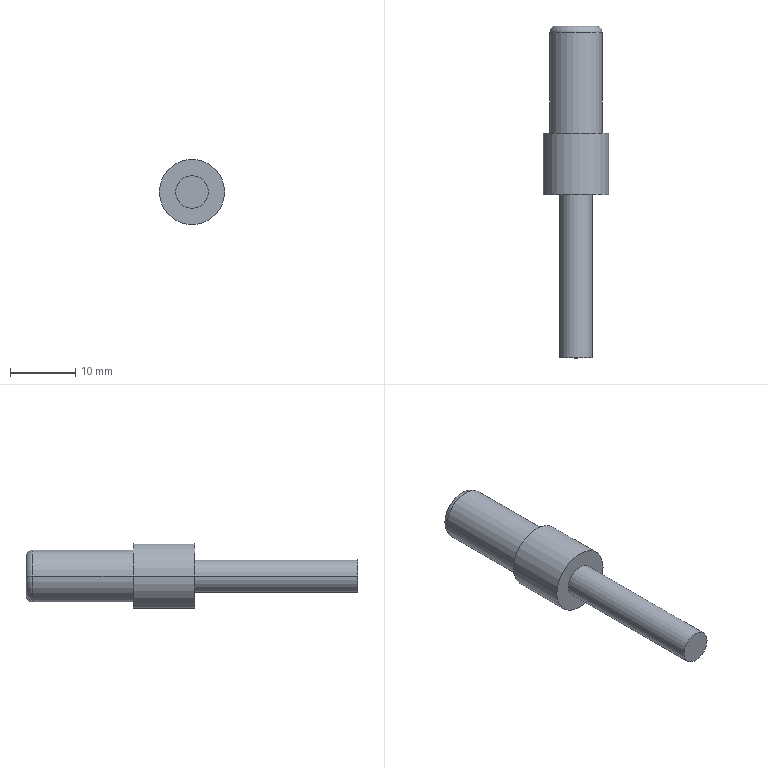Part | STEP file | 11-NEZIPART_CLDM5-25-B11 | 1 solid | 19 faces | box 10 x 50.8 x 10 mm | volume 2025 mm3 | plane 11 | cylinder 6 | torus 2 | commonest cylinder face diameters 5 x2 8 x2 10 x2
STEP:
#1=CARTESIAN_POINT('',(-2.5,-25.,0.));
#2=VERTEX_POINT('',#1);
#3=CARTESIAN_POINT('',(2.5,-25.,0.));
#4=VERTEX_POINT('',#3);
#5=CARTESIAN_POINT('',(0.,-25.,0.));
#6=DIRECTION('',(0.,1.,0.));
#7=DIRECTION('',(-1.,0.,0.));
#8=AXIS2_PLACEMENT_3D('',#5,#6,#7);
#9=CIRCLE('',#8,2.5);
#10=EDGE_CURVE('',#2,#4,#9,.T.);
#11=ORIENTED_EDGE('',*,*,#10,.T.);
#12=CARTESIAN_POINT('',(2.5,0.,0.));
#13=VERTEX_POINT('',#12);
#14=CARTESIAN_POINT('',(2.5,25.8,0.));
#15=DIRECTION('',(0.,1.,0.));
#16=VECTOR('',#15,1000.);
#17=LINE('',#14,#16);
#18=EDGE_CURVE('',#4,#13,#17,.T.);
#19=ORIENTED_EDGE('',*,*,#18,.T.);
#20=CARTESIAN_POINT('',(-2.5,0.,0.));
#21=VERTEX_POINT('',#20);
#22=CARTESIAN_POINT('',(0.,0.,0.));
#23=DIRECTION('',(0.,1.,0.));
#24=DIRECTION('',(-1.,0.,0.));
#25=AXIS2_PLACEMENT_3D('',#22,#23,#24);
#26=CIRCLE('',#25,2.5);
#27=EDGE_CURVE('',#21,#13,#26,.T.);
#28=ORIENTED_EDGE('',*,*,#27,.F.);
#29=CARTESIAN_POINT('',(-2.5,25.8,0.));
#30=DIRECTION('',(0.,1.,0.));
#31=VECTOR('',#30,1000.);
#32=LINE('',#29,#31);
#33=EDGE_CURVE('',#2,#21,#32,.T.);
#34=ORIENTED_EDGE('',*,*,#33,.F.);
#35=EDGE_LOOP('',(#11,#19,#28,#34));
#36=FACE_OUTER_BOUND('',#35,.T.);
#37=CARTESIAN_POINT('',(0.,25.8,0.));
#38=DIRECTION('',(0.,1.,0.));
#39=DIRECTION('',(-1.,0.,0.));
#40=AXIS2_PLACEMENT_3D('',#37,#38,#39);
#41=CYLINDRICAL_SURFACE('',#40,2.5);
#42=ADVANCED_FACE('',(#36),#41,.T.);
#43=CARTESIAN_POINT('',(-4.,24.8,0.));
#44=VERTEX_POINT('',#43);
#45=CARTESIAN_POINT('',(4.,24.8,0.));
#46=VERTEX_POINT('',#45);
#47=CARTESIAN_POINT('',(0.,24.8,0.));
#48=DIRECTION('',(0.,1.,0.));
#49=DIRECTION('',(-1.,0.,0.));
#50=AXIS2_PLACEMENT_3D('',#47,#48,#49);
#51=CIRCLE('',#50,4.);
#52=EDGE_CURVE('',#44,#46,#51,.T.);
#53=ORIENTED_EDGE('',*,*,#52,.T.);
#54=CARTESIAN_POINT('',(3.,25.8,0.));
#55=VERTEX_POINT('',#54);
#56=CARTESIAN_POINT('',(3.,24.8,0.));
#57=DIRECTION('',(0.,0.,1.));
#58=DIRECTION('',(1.,0.,0.));
#59=AXIS2_PLACEMENT_3D('',#56,#57,#58);
#60=CIRCLE('',#59,1.);
#61=EDGE_CURVE('',#46,#55,#60,.T.);
#62=ORIENTED_EDGE('',*,*,#61,.T.);
#63=CARTESIAN_POINT('',(-3.,25.8,0.));
#64=VERTEX_POINT('',#63);
#65=CARTESIAN_POINT('',(0.,25.8,0.));
#66=DIRECTION('',(0.,1.,0.));
#67=DIRECTION('',(-1.,0.,0.));
#68=AXIS2_PLACEMENT_3D('',#65,#66,#67);
#69=CIRCLE('',#68,3.);
#70=EDGE_CURVE('',#64,#55,#69,.T.);
#71=ORIENTED_EDGE('',*,*,#70,.F.);
#72=CARTESIAN_POINT('',(-3.,24.8,0.));
#73=DIRECTION('',(0.,0.,-1.));
#74=DIRECTION('',(-1.,0.,0.));
#75=AXIS2_PLACEMENT_3D('',#72,#73,#74);
#76=CIRCLE('',#75,1.);
#77=EDGE_CURVE('',#44,#64,#76,.T.);
#78=ORIENTED_EDGE('',*,*,#77,.F.);
#79=EDGE_LOOP('',(#53,#62,#71,#78));
#80=FACE_OUTER_BOUND('',#79,.T.);
#81=CARTESIAN_POINT('',(0.,24.8,0.));
#82=DIRECTION('',(0.,1.,0.));
#83=DIRECTION('',(-1.,0.,0.));
#84=AXIS2_PLACEMENT_3D('',#81,#82,#83);
#85=TOROIDAL_SURFACE('',#84,3.,1.);
#86=ADVANCED_FACE('',(#80),#85,.T.);
#87=CARTESIAN_POINT('',(-4.,9.4,0.));
#88=VERTEX_POINT('',#87);
#89=CARTESIAN_POINT('',(4.,9.4,0.));
#90=VERTEX_POINT('',#89);
#91=CARTESIAN_POINT('',(0.,9.4,0.));
#92=DIRECTION('',(0.,1.,0.));
#93=DIRECTION('',(-1.,0.,0.));
#94=AXIS2_PLACEMENT_3D('',#91,#92,#93);
#95=CIRCLE('',#94,4.);
#96=EDGE_CURVE('',#88,#90,#95,.T.);
#97=ORIENTED_EDGE('',*,*,#96,.T.);
#98=CARTESIAN_POINT('',(4.,25.8,0.));
#99=DIRECTION('',(0.,1.,0.));
#100=VECTOR('',#99,1000.);
#101=LINE('',#98,#100);
#102=EDGE_CURVE('',#90,#46,#101,.T.);
#103=ORIENTED_EDGE('',*,*,#102,.T.);
#104=ORIENTED_EDGE('',*,*,#52,.F.);
#105=CARTESIAN_POINT('',(-4.,25.8,0.));
#106=DIRECTION('',(0.,1.,0.));
#107=VECTOR('',#106,1000.);
#108=LINE('',#105,#107);
#109=EDGE_CURVE('',#88,#44,#108,.T.);
#110=ORIENTED_EDGE('',*,*,#109,.F.);
#111=EDGE_LOOP('',(#97,#103,#104,#110));
#112=FACE_OUTER_BOUND('',#111,.T.);
#113=CARTESIAN_POINT('',(0.,25.8,0.));
#114=DIRECTION('',(0.,1.,0.));
#115=DIRECTION('',(-1.,0.,0.));
#116=AXIS2_PLACEMENT_3D('',#113,#114,#115);
#117=CYLINDRICAL_SURFACE('',#116,4.);
#118=ADVANCED_FACE('',(#112),#117,.T.);
#119=CARTESIAN_POINT('',(-5.,0.,0.));
#120=VERTEX_POINT('',#119);
#121=CARTESIAN_POINT('',(5.,0.,0.));
#122=VERTEX_POINT('',#121);
#123=CARTESIAN_POINT('',(0.,0.,0.));
#124=DIRECTION('',(0.,1.,0.));
#125=DIRECTION('',(-1.,0.,0.));
#126=AXIS2_PLACEMENT_3D('',#123,#124,#125);
#127=CIRCLE('',#126,5.);
#128=EDGE_CURVE('',#120,#122,#127,.T.);
#129=ORIENTED_EDGE('',*,*,#128,.T.);
#130=CARTESIAN_POINT('',(5.,9.4,0.));
#131=VERTEX_POINT('',#130);
#132=CARTESIAN_POINT('',(5.,25.8,0.));
#133=DIRECTION('',(0.,1.,0.));
#134=VECTOR('',#133,1000.);
#135=LINE('',#132,#134);
#136=EDGE_CURVE('',#122,#131,#135,.T.);
#137=ORIENTED_EDGE('',*,*,#136,.T.);
#138=CARTESIAN_POINT('',(-5.,9.4,0.));
#139=VERTEX_POINT('',#138);
#140=CARTESIAN_POINT('',(0.,9.4,0.));
#141=DIRECTION('',(0.,1.,0.));
#142=DIRECTION('',(-1.,0.,0.));
#143=AXIS2_PLACEMENT_3D('',#140,#141,#142);
#144=CIRCLE('',#143,5.);
#145=EDGE_CURVE('',#139,#131,#144,.T.);
#146=ORIENTED_EDGE('',*,*,#145,.F.);
#147=CARTESIAN_POINT('',(-5.,25.8,0.));
#148=DIRECTION('',(0.,1.,0.));
#149=VECTOR('',#148,1000.);
#150=LINE('',#147,#149);
#151=EDGE_CURVE('',#120,#139,#150,.T.);
#152=ORIENTED_EDGE('',*,*,#151,.F.);
#153=EDGE_LOOP('',(#129,#137,#146,#152));
#154=FACE_OUTER_BOUND('',#153,.T.);
#155=CARTESIAN_POINT('',(0.,25.8,0.));
#156=DIRECTION('',(0.,1.,0.));
#157=DIRECTION('',(-1.,0.,0.));
#158=AXIS2_PLACEMENT_3D('',#155,#156,#157);
#159=CYLINDRICAL_SURFACE('',#158,5.);
#160=ADVANCED_FACE('',(#154),#159,.T.);
#161=ORIENTED_EDGE('',*,*,#128,.F.);
#162=CARTESIAN_POINT('',(0.,0.,0.));
#163=DIRECTION('',(0.,1.,0.));
#164=DIRECTION('',(-1.,0.,0.));
#165=AXIS2_PLACEMENT_3D('',#162,#163,#164);
#166=CIRCLE('',#165,5.);
#167=EDGE_CURVE('',#122,#120,#166,.T.);
#168=ORIENTED_EDGE('',*,*,#167,.F.);
#169=EDGE_LOOP('',(#161,#168));
#170=FACE_OUTER_BOUND('',#169,.T.);
#171=ORIENTED_EDGE('',*,*,#27,.T.);
#172=CARTESIAN_POINT('',(0.,0.,0.));
#173=DIRECTION('',(0.,1.,0.));
#174=DIRECTION('',(-1.,0.,0.));
#175=AXIS2_PLACEMENT_3D('',#172,#173,#174);
#176=CIRCLE('',#175,2.5);
#177=EDGE_CURVE('',#13,#21,#176,.T.);
#178=ORIENTED_EDGE('',*,*,#177,.T.);
#179=EDGE_LOOP('',(#171,#178));
#180=FACE_BOUND('',#179,.T.);
#181=CARTESIAN_POINT('',(2.5,0.,0.));
#182=DIRECTION('',(0.,1.,0.));
#183=DIRECTION('',(-1.,0.,0.));
#184=AXIS2_PLACEMENT_3D('',#181,#182,#183);
#185=PLANE('',#184);
#186=ADVANCED_FACE('',(#170,#180),#185,.F.);
#187=ORIENTED_EDGE('',*,*,#136,.F.);
#188=ORIENTED_EDGE('',*,*,#167,.T.);
#189=ORIENTED_EDGE('',*,*,#151,.T.);
#190=CARTESIAN_POINT('',(0.,9.4,0.));
#191=DIRECTION('',(0.,1.,0.));
#192=DIRECTION('',(-1.,0.,0.));
#193=AXIS2_PLACEMENT_3D('',#190,#191,#192);
#194=CIRCLE('',#193,5.);
#195=EDGE_CURVE('',#131,#139,#194,.T.);
#196=ORIENTED_EDGE('',*,*,#195,.F.);
#197=EDGE_LOOP('',(#187,#188,#189,#196));
#198=FACE_OUTER_BOUND('',#197,.T.);
#199=CARTESIAN_POINT('',(0.,25.8,0.));
#200=DIRECTION('',(0.,1.,0.));
#201=DIRECTION('',(-1.,0.,0.));
#202=AXIS2_PLACEMENT_3D('',#199,#200,#201);
#203=CYLINDRICAL_SURFACE('',#202,5.);
#204=ADVANCED_FACE('',(#198),#203,.T.);
#205=ORIENTED_EDGE('',*,*,#96,.F.);
#206=CARTESIAN_POINT('',(0.,9.4,0.));
#207=DIRECTION('',(0.,1.,0.));
#208=DIRECTION('',(-1.,0.,0.));
#209=AXIS2_PLACEMENT_3D('',#206,#207,#208);
#210=CIRCLE('',#209,4.);
#211=EDGE_CURVE('',#90,#88,#210,.T.);
#212=ORIENTED_EDGE('',*,*,#211,.F.);
#213=EDGE_LOOP('',(#205,#212));
#214=FACE_BOUND('',#213,.T.);
#215=ORIENTED_EDGE('',*,*,#145,.T.);
#216=ORIENTED_EDGE('',*,*,#195,.T.);
#217=EDGE_LOOP('',(#215,#216));
#218=FACE_OUTER_BOUND('',#217,.T.);
#219=CARTESIAN_POINT('',(5.,9.4,0.));
#220=DIRECTION('',(0.,-1.,0.));
#221=DIRECTION('',(1.,0.,0.));
#222=AXIS2_PLACEMENT_3D('',#219,#220,#221);
#223=PLANE('',#222);
#224=ADVANCED_FACE('',(#214,#218),#223,.F.);
#225=ORIENTED_EDGE('',*,*,#102,.F.);
#226=ORIENTED_EDGE('',*,*,#211,.T.);
#227=ORIENTED_EDGE('',*,*,#109,.T.);
#228=CARTESIAN_POINT('',(0.,24.8,0.));
#229=DIRECTION('',(0.,1.,0.));
#230=DIRECTION('',(-1.,0.,0.));
#231=AXIS2_PLACEMENT_3D('',#228,#229,#230);
#232=CIRCLE('',#231,4.);
#233=EDGE_CURVE('',#46,#44,#232,.T.);
#234=ORIENTED_EDGE('',*,*,#233,.F.);
#235=EDGE_LOOP('',(#225,#226,#227,#234));
#236=FACE_OUTER_BOUND('',#235,.T.);
#237=CARTESIAN_POINT('',(0.,25.8,0.));
#238=DIRECTION('',(0.,1.,0.));
#239=DIRECTION('',(-1.,0.,0.));
#240=AXIS2_PLACEMENT_3D('',#237,#238,#239);
#241=CYLINDRICAL_SURFACE('',#240,4.);
#242=ADVANCED_FACE('',(#236),#241,.T.);
#243=ORIENTED_EDGE('',*,*,#61,.F.);
#244=ORIENTED_EDGE('',*,*,#233,.T.);
#245=ORIENTED_EDGE('',*,*,#77,.T.);
#246=CARTESIAN_POINT('',(0.,25.8,0.));
#247=DIRECTION('',(0.,1.,0.));
#248=DIRECTION('',(-1.,0.,0.));
#249=AXIS2_PLACEMENT_3D('',#246,#247,#248);
#250=CIRCLE('',#249,3.);
#251=EDGE_CURVE('',#55,#64,#250,.T.);
#252=ORIENTED_EDGE('',*,*,#251,.F.);
#253=EDGE_LOOP('',(#243,#244,#245,#252));
#254=FACE_OUTER_BOUND('',#253,.T.);
#255=CARTESIAN_POINT('',(0.,24.8,0.));
#256=DIRECTION('',(0.,1.,0.));
#257=DIRECTION('',(-1.,0.,0.));
#258=AXIS2_PLACEMENT_3D('',#255,#256,#257);
#259=TOROIDAL_SURFACE('',#258,3.,1.);
#260=ADVANCED_FACE('',(#254),#259,.T.);
#261=CARTESIAN_POINT('',(0.,25.8,-1.732));
#262=VERTEX_POINT('',#261);
#263=CARTESIAN_POINT('',(-1.5,25.8,-0.866));
#264=VERTEX_POINT('',#263);
#265=CARTESIAN_POINT('',(0.,25.8,-1.732));
#266=DIRECTION('',(-0.866,0.,0.5));
#267=VECTOR('',#266,1000.);
#268=LINE('',#265,#267);
#269=EDGE_CURVE('',#262,#264,#268,.T.);
#270=ORIENTED_EDGE('',*,*,#269,.F.);
#271=CARTESIAN_POINT('',(1.5,25.8,-0.866));
#272=VERTEX_POINT('',#271);
#273=CARTESIAN_POINT('',(1.5,25.8,-0.866));
#274=DIRECTION('',(-0.866,0.,-0.5));
#275=VECTOR('',#274,1000.);
#276=LINE('',#273,#275);
#277=EDGE_CURVE('',#272,#262,#276,.T.);
#278=ORIENTED_EDGE('',*,*,#277,.F.);
#279=CARTESIAN_POINT('',(1.5,25.8,0.866));
#280=VERTEX_POINT('',#279);
#281=CARTESIAN_POINT('',(1.5,25.8,0.866));
#282=DIRECTION('',(0.,0.,-1.));
#283=VECTOR('',#282,1000.);
#284=LINE('',#281,#283);
#285=EDGE_CURVE('',#280,#272,#284,.T.);
#286=ORIENTED_EDGE('',*,*,#285,.F.);
#287=CARTESIAN_POINT('',(0.,25.8,1.732));
#288=VERTEX_POINT('',#287);
#289=CARTESIAN_POINT('',(0.,25.8,1.732));
#290=DIRECTION('',(0.866,0.,-0.5));
#291=VECTOR('',#290,1000.);
#292=LINE('',#289,#291);
#293=EDGE_CURVE('',#288,#280,#292,.T.);
#294=ORIENTED_EDGE('',*,*,#293,.F.);
#295=CARTESIAN_POINT('',(-1.5,25.8,0.866));
#296=VERTEX_POINT('',#295);
#297=CARTESIAN_POINT('',(-1.5,25.8,0.866));
#298=DIRECTION('',(0.866,0.,0.5));
#299=VECTOR('',#298,1000.);
#300=LINE('',#297,#299);
#301=EDGE_CURVE('',#296,#288,#300,.T.);
#302=ORIENTED_EDGE('',*,*,#301,.F.);
#303=CARTESIAN_POINT('',(-1.5,25.8,-0.866));
#304=DIRECTION('',(0.,0.,1.));
#305=VECTOR('',#304,1000.);
#306=LINE('',#303,#305);
#307=EDGE_CURVE('',#264,#296,#306,.T.);
#308=ORIENTED_EDGE('',*,*,#307,.F.);
#309=EDGE_LOOP('',(#270,#278,#286,#294,#302,#308));
#310=FACE_BOUND('',#309,.T.);
#311=ORIENTED_EDGE('',*,*,#70,.T.);
#312=ORIENTED_EDGE('',*,*,#251,.T.);
#313=EDGE_LOOP('',(#311,#312));
#314=FACE_OUTER_BOUND('',#313,.T.);
#315=CARTESIAN_POINT('',(3.,25.8,0.));
#316=DIRECTION('',(0.,-1.,0.));
#317=DIRECTION('',(1.,0.,0.));
#318=AXIS2_PLACEMENT_3D('',#315,#316,#317);
#319=PLANE('',#318);
#320=ADVANCED_FACE('',(#310,#314),#319,.F.);
#321=ORIENTED_EDGE('',*,*,#10,.F.);
#322=CARTESIAN_POINT('',(0.,-25.,0.));
#323=DIRECTION('',(0.,1.,0.));
#324=DIRECTION('',(-1.,0.,0.));
#325=AXIS2_PLACEMENT_3D('',#322,#323,#324);
#326=CIRCLE('',#325,2.5);
#327=EDGE_CURVE('',#4,#2,#326,.T.);
#328=ORIENTED_EDGE('',*,*,#327,.F.);
#329=EDGE_LOOP('',(#321,#328));
#330=FACE_OUTER_BOUND('',#329,.T.);
#331=CARTESIAN_POINT('',(0.,-25.,0.));
#332=DIRECTION('',(0.,1.,0.));
#333=DIRECTION('',(-1.,0.,0.));
#334=AXIS2_PLACEMENT_3D('',#331,#332,#333);
#335=PLANE('',#334);
#336=ADVANCED_FACE('',(#330),#335,.F.);
#337=ORIENTED_EDGE('',*,*,#18,.F.);
#338=ORIENTED_EDGE('',*,*,#327,.T.);
#339=ORIENTED_EDGE('',*,*,#33,.T.);
#340=ORIENTED_EDGE('',*,*,#177,.F.);
#341=EDGE_LOOP('',(#337,#338,#339,#340));
#342=FACE_OUTER_BOUND('',#341,.T.);
#343=CARTESIAN_POINT('',(0.,25.8,0.));
#344=DIRECTION('',(0.,1.,0.));
#345=DIRECTION('',(-1.,0.,0.));
#346=AXIS2_PLACEMENT_3D('',#343,#344,#345);
#347=CYLINDRICAL_SURFACE('',#346,2.5);
#348=ADVANCED_FACE('',(#342),#347,.T.);
#349=ORIENTED_EDGE('',*,*,#277,.T.);
#350=CARTESIAN_POINT('',(0.,22.8,-1.732));
#351=VERTEX_POINT('',#350);
#352=CARTESIAN_POINT('',(0.,22.8,-1.732));
#353=DIRECTION('',(0.,1.,0.));
#354=VECTOR('',#353,1000.);
#355=LINE('',#352,#354);
#356=EDGE_CURVE('',#351,#262,#355,.T.);
#357=ORIENTED_EDGE('',*,*,#356,.F.);
#358=CARTESIAN_POINT('',(1.5,22.8,-0.866));
#359=VERTEX_POINT('',#358);
#360=CARTESIAN_POINT('',(1.5,22.8,-0.866));
#361=DIRECTION('',(-0.866,0.,-0.5));
#362=VECTOR('',#361,1000.);
#363=LINE('',#360,#362);
#364=EDGE_CURVE('',#359,#351,#363,.T.);
#365=ORIENTED_EDGE('',*,*,#364,.F.);
#366=CARTESIAN_POINT('',(1.5,22.8,-0.866));
#367=DIRECTION('',(0.,1.,0.));
#368=VECTOR('',#367,1000.);
#369=LINE('',#366,#368);
#370=EDGE_CURVE('',#359,#272,#369,.T.);
#371=ORIENTED_EDGE('',*,*,#370,.T.);
#372=EDGE_LOOP('',(#349,#357,#365,#371));
#373=FACE_OUTER_BOUND('',#372,.T.);
#374=CARTESIAN_POINT('',(1.5,22.8,-0.866));
#375=DIRECTION('',(0.5,0.,-0.866));
#376=DIRECTION('',(-0.866,0.,-0.5));
#377=AXIS2_PLACEMENT_3D('',#374,#375,#376);
#378=PLANE('',#377);
#379=ADVANCED_FACE('',(#373),#378,.F.);
#380=ORIENTED_EDGE('',*,*,#285,.T.);
#381=ORIENTED_EDGE('',*,*,#370,.F.);
#382=CARTESIAN_POINT('',(1.5,22.8,0.866));
#383=VERTEX_POINT('',#382);
#384=CARTESIAN_POINT('',(1.5,22.8,0.866));
#385=DIRECTION('',(0.,0.,-1.));
#386=VECTOR('',#385,1000.);
#387=LINE('',#384,#386);
#388=EDGE_CURVE('',#383,#359,#387,.T.);
#389=ORIENTED_EDGE('',*,*,#388,.F.);
#390=CARTESIAN_POINT('',(1.5,22.8,0.866));
#391=DIRECTION('',(0.,1.,0.));
#392=VECTOR('',#391,1000.);
#393=LINE('',#390,#392);
#394=EDGE_CURVE('',#383,#280,#393,.T.);
#395=ORIENTED_EDGE('',*,*,#394,.T.);
#396=EDGE_LOOP('',(#380,#381,#389,#395));
#397=FACE_OUTER_BOUND('',#396,.T.);
#398=CARTESIAN_POINT('',(1.5,22.8,0.866));
#399=DIRECTION('',(1.,0.,0.));
#400=DIRECTION('',(0.,0.,-1.));
#401=AXIS2_PLACEMENT_3D('',#398,#399,#400);
#402=PLANE('',#401);
#403=ADVANCED_FACE('',(#397),#402,.F.);
#404=ORIENTED_EDGE('',*,*,#293,.T.);
#405=ORIENTED_EDGE('',*,*,#394,.F.);
#406=CARTESIAN_POINT('',(0.,22.8,1.732));
#407=VERTEX_POINT('',#406);
#408=CARTESIAN_POINT('',(0.,22.8,1.732));
#409=DIRECTION('',(0.866,0.,-0.5));
#410=VECTOR('',#409,1000.);
#411=LINE('',#408,#410);
#412=EDGE_CURVE('',#407,#383,#411,.T.);
#413=ORIENTED_EDGE('',*,*,#412,.F.);
#414=CARTESIAN_POINT('',(0.,22.8,1.732));
#415=DIRECTION('',(0.,1.,0.));
#416=VECTOR('',#415,1000.);
#417=LINE('',#414,#416);
#418=EDGE_CURVE('',#407,#288,#417,.T.);
#419=ORIENTED_EDGE('',*,*,#418,.T.);
#420=EDGE_LOOP('',(#404,#405,#413,#419));
#421=FACE_OUTER_BOUND('',#420,.T.);
#422=CARTESIAN_POINT('',(0.,22.8,1.732));
#423=DIRECTION('',(0.5,0.,0.866));
#424=DIRECTION('',(0.866,0.,-0.5));
#425=AXIS2_PLACEMENT_3D('',#422,#423,#424);
#426=PLANE('',#425);
#427=ADVANCED_FACE('',(#421),#426,.F.);
#428=ORIENTED_EDGE('',*,*,#301,.T.);
#429=ORIENTED_EDGE('',*,*,#418,.F.);
#430=CARTESIAN_POINT('',(-1.5,22.8,0.866));
#431=VERTEX_POINT('',#430);
#432=CARTESIAN_POINT('',(-1.5,22.8,0.866));
#433=DIRECTION('',(0.866,0.,0.5));
#434=VECTOR('',#433,1000.);
#435=LINE('',#432,#434);
#436=EDGE_CURVE('',#431,#407,#435,.T.);
#437=ORIENTED_EDGE('',*,*,#436,.F.);
#438=CARTESIAN_POINT('',(-1.5,22.8,0.866));
#439=DIRECTION('',(0.,1.,0.));
#440=VECTOR('',#439,1000.);
#441=LINE('',#438,#440);
#442=EDGE_CURVE('',#431,#296,#441,.T.);
#443=ORIENTED_EDGE('',*,*,#442,.T.);
#444=EDGE_LOOP('',(#428,#429,#437,#443));
#445=FACE_OUTER_BOUND('',#444,.T.);
#446=CARTESIAN_POINT('',(-1.5,22.8,0.866));
#447=DIRECTION('',(-0.5,0.,0.866));
#448=DIRECTION('',(0.866,0.,0.5));
#449=AXIS2_PLACEMENT_3D('',#446,#447,#448);
#450=PLANE('',#449);
#451=ADVANCED_FACE('',(#445),#450,.F.);
#452=ORIENTED_EDGE('',*,*,#307,.T.);
#453=ORIENTED_EDGE('',*,*,#442,.F.);
#454=CARTESIAN_POINT('',(-1.5,22.8,-0.866));
#455=VERTEX_POINT('',#454);
#456=CARTESIAN_POINT('',(-1.5,22.8,-0.866));
#457=DIRECTION('',(0.,0.,1.));
#458=VECTOR('',#457,1000.);
#459=LINE('',#456,#458);
#460=EDGE_CURVE('',#455,#431,#459,.T.);
#461=ORIENTED_EDGE('',*,*,#460,.F.);
#462=CARTESIAN_POINT('',(-1.5,22.8,-0.866));
#463=DIRECTION('',(0.,1.,0.));
#464=VECTOR('',#463,1000.);
#465=LINE('',#462,#464);
#466=EDGE_CURVE('',#455,#264,#465,.T.);
#467=ORIENTED_EDGE('',*,*,#466,.T.);
#468=EDGE_LOOP('',(#452,#453,#461,#467));
#469=FACE_OUTER_BOUND('',#468,.T.);
#470=CARTESIAN_POINT('',(-1.5,22.8,-0.866));
#471=DIRECTION('',(-1.,0.,0.));
#472=DIRECTION('',(0.,0.,1.));
#473=AXIS2_PLACEMENT_3D('',#470,#471,#472);
#474=PLANE('',#473);
#475=ADVANCED_FACE('',(#469),#474,.F.);
#476=ORIENTED_EDGE('',*,*,#269,.T.);
#477=ORIENTED_EDGE('',*,*,#466,.F.);
#478=CARTESIAN_POINT('',(0.,22.8,-1.732));
#479=DIRECTION('',(-0.866,0.,0.5));
#480=VECTOR('',#479,1000.);
#481=LINE('',#478,#480);
#482=EDGE_CURVE('',#351,#455,#481,.T.);
#483=ORIENTED_EDGE('',*,*,#482,.F.);
#484=ORIENTED_EDGE('',*,*,#356,.T.);
#485=EDGE_LOOP('',(#476,#477,#483,#484));
#486=FACE_OUTER_BOUND('',#485,.T.);
#487=CARTESIAN_POINT('',(0.,22.8,-1.732));
#488=DIRECTION('',(-0.5,0.,-0.866));
#489=DIRECTION('',(-0.866,0.,0.5));
#490=AXIS2_PLACEMENT_3D('',#487,#488,#489);
#491=PLANE('',#490);
#492=ADVANCED_FACE('',(#486),#491,.F.);
#493=ORIENTED_EDGE('',*,*,#364,.T.);
#494=ORIENTED_EDGE('',*,*,#482,.T.);
#495=ORIENTED_EDGE('',*,*,#460,.T.);
#496=ORIENTED_EDGE('',*,*,#436,.T.);
#497=ORIENTED_EDGE('',*,*,#412,.T.);
#498=ORIENTED_EDGE('',*,*,#388,.T.);
#499=EDGE_LOOP('',(#493,#494,#495,#496,#497,#498));
#500=FACE_OUTER_BOUND('',#499,.T.);
#501=CARTESIAN_POINT('',(0.,22.8,0.));
#502=DIRECTION('',(0.,1.,0.));
#503=DIRECTION('',(0.,0.,1.));
#504=AXIS2_PLACEMENT_3D('',#501,#502,#503);
#505=PLANE('',#504);
#506=ADVANCED_FACE('',(#500),#505,.T.);
#507=CLOSED_SHELL('',(#42,#86,#118,#160,#186,#204,#224,#242,#260,#320,#336,#348,#379,#403,#427,#451,#475,#492,#506));
#508=MANIFOLD_SOLID_BREP('',#507);
#509=CARTESIAN_POINT('',(0.,0.,0.));
#510=DIRECTION('',(0.,0.,1.));
#511=DIRECTION('',(1.,0.,0.));
#512=AXIS2_PLACEMENT_3D('',#509,#510,#511);
#513=(LENGTH_UNIT()NAMED_UNIT(*)SI_UNIT(.MILLI.,.METRE.));
#514=UNCERTAINTY_MEASURE_WITH_UNIT(LENGTH_MEASURE(0.00001),#513,'','');
#515=(NAMED_UNIT(*)PLANE_ANGLE_UNIT()SI_UNIT($,.RADIAN.));
#516=(NAMED_UNIT(*)SI_UNIT($,.STERADIAN.)SOLID_ANGLE_UNIT());
#517=(GEOMETRIC_REPRESENTATION_CONTEXT(3)GLOBAL_UNCERTAINTY_ASSIGNED_CONTEXT((#514))GLOBAL_UNIT_ASSIGNED_CONTEXT((#513,#515,#516))REPRESENTATION_CONTEXT('',''));
#518=ADVANCED_BREP_SHAPE_REPRESENTATION('',(#508,#512),#517);